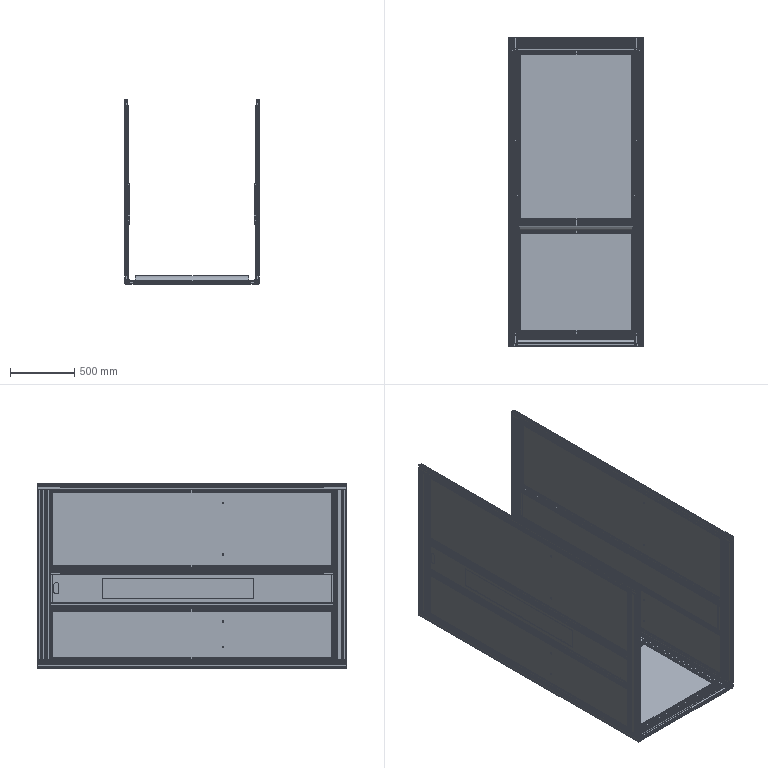Part | SolidWorks | features ReferencePattern 10, MirrorCompFeat 5 | 149 solids | 5267 faces | volume 215809773 mm3 | plane 3402 | cylinder 1865 | commonest cylinder face diameters 1.1 x240 3.6 x204 8.5 x204 5.8 x198 0.4 x127 0.6 x112